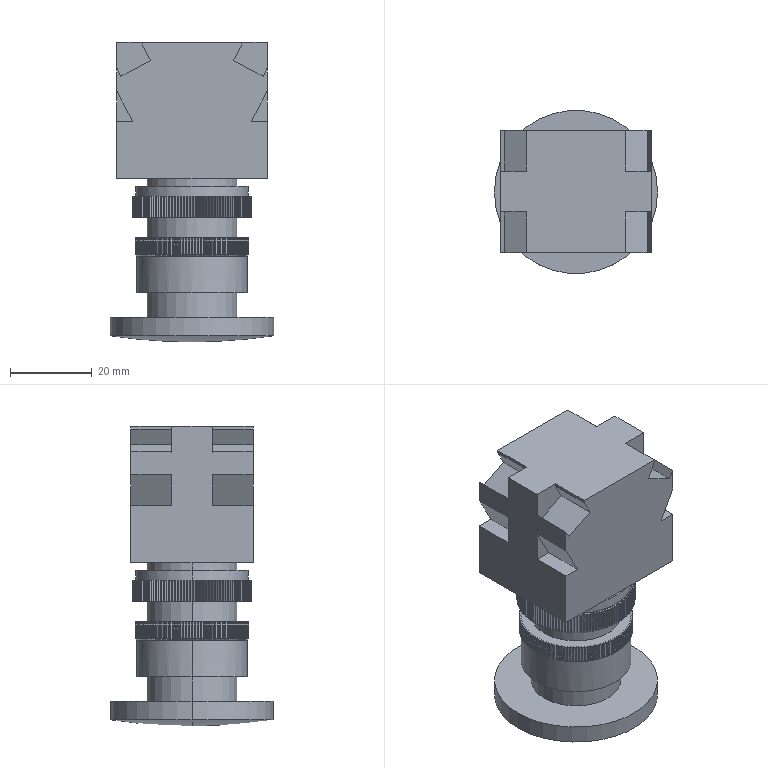Part | SolidWorks | features ICE 8, CirPattern 2, Chamfer 1, Extrusion 1, MirrorPattern 1, Revolution 1 | 1 solid | 1017 faces | box 40 x 40 x 73.5 mm | volume 58670 mm3 | plane 643 | cylinder 252 | cone 120 | sphere 2 | commonest cylinder face diameters 27.8 x120 29 x120 22 x6 27 x2 27.5 x2 40 x2